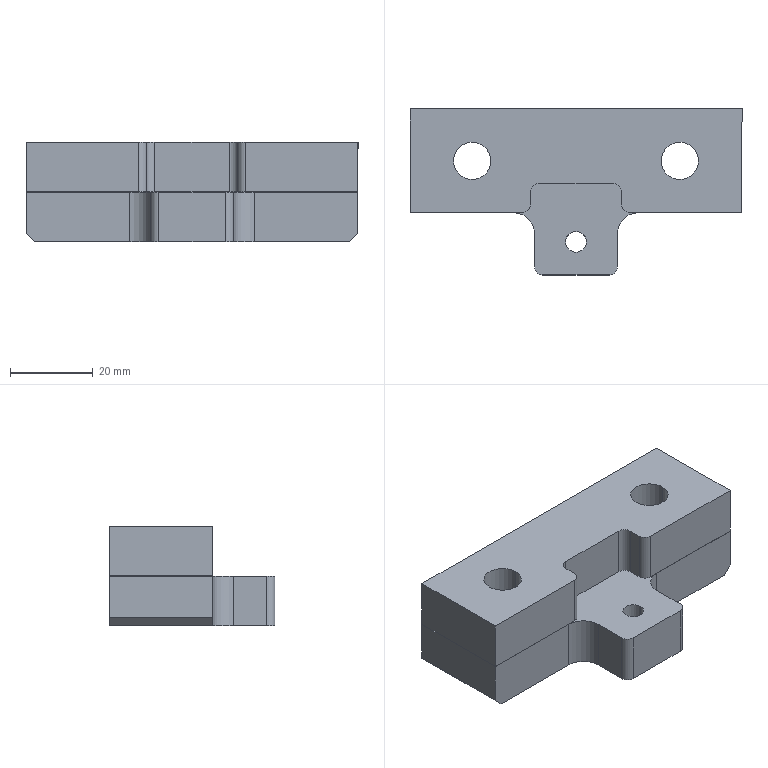Part | SolidWorks | features ICE 5, Fillet 3, HoleWzd 2, Chamfer 1, Extrusion 1 | 2 solids | 40 faces | box 80 x 40 x 24 mm | volume 46437 mm3 | plane 22 | cylinder 18 | commonest cylinder face diameters 9 x8 4 x6 5 x2 10 x2
STEP:
#1=CARTESIAN_POINT('',(60.5,7.5,-12.));
#2=VERTEX_POINT('',#1);
#3=CARTESIAN_POINT('',(69.5,7.5,-12.));
#4=VERTEX_POINT('',#3);
#5=CARTESIAN_POINT('',(65.,7.5,-12.));
#6=DIRECTION('',(0.,0.,1.));
#7=DIRECTION('',(-1.,0.,0.));
#8=AXIS2_PLACEMENT_3D('',#5,#6,#7);
#9=CIRCLE('',#8,4.5);
#10=EDGE_CURVE('',#2,#4,#9,.T.);
#11=ORIENTED_EDGE('',*,*,#10,.T.);
#12=CARTESIAN_POINT('',(69.5,7.5,-24.));
#13=VERTEX_POINT('',#12);
#14=CARTESIAN_POINT('',(69.5,7.5,-24.));
#15=DIRECTION('',(0.,0.,-1.));
#16=VECTOR('',#15,1000.);
#17=LINE('',#14,#16);
#18=EDGE_CURVE('',#4,#13,#17,.T.);
#19=ORIENTED_EDGE('',*,*,#18,.T.);
#20=CARTESIAN_POINT('',(60.5,7.5,-24.));
#21=VERTEX_POINT('',#20);
#22=CARTESIAN_POINT('',(65.,7.5,-24.));
#23=DIRECTION('',(0.,0.,-1.));
#24=DIRECTION('',(-1.,0.,0.));
#25=AXIS2_PLACEMENT_3D('',#22,#23,#24);
#26=CIRCLE('',#25,4.5);
#27=EDGE_CURVE('',#13,#21,#26,.T.);
#28=ORIENTED_EDGE('',*,*,#27,.T.);
#29=CARTESIAN_POINT('',(60.5,7.5,-24.));
#30=DIRECTION('',(0.,0.,-1.));
#31=VECTOR('',#30,1000.);
#32=LINE('',#29,#31);
#33=EDGE_CURVE('',#2,#21,#32,.T.);
#34=ORIENTED_EDGE('',*,*,#33,.F.);
#35=EDGE_LOOP('',(#11,#19,#28,#34));
#36=FACE_OUTER_BOUND('',#35,.T.);
#37=CARTESIAN_POINT('',(65.,7.5,-24.));
#38=DIRECTION('',(0.,0.,-1.));
#39=DIRECTION('',(-1.,0.,0.));
#40=AXIS2_PLACEMENT_3D('',#37,#38,#39);
#41=CYLINDRICAL_SURFACE('',#40,4.5);
#42=ADVANCED_FACE('',(#36),#41,.F.);
#43=CARTESIAN_POINT('',(10.5,7.5,-12.));
#44=VERTEX_POINT('',#43);
#45=CARTESIAN_POINT('',(19.5,7.5,-12.));
#46=VERTEX_POINT('',#45);
#47=CARTESIAN_POINT('',(15.,7.5,-12.));
#48=DIRECTION('',(0.,0.,1.));
#49=DIRECTION('',(-1.,0.,0.));
#50=AXIS2_PLACEMENT_3D('',#47,#48,#49);
#51=CIRCLE('',#50,4.5);
#52=EDGE_CURVE('',#44,#46,#51,.T.);
#53=ORIENTED_EDGE('',*,*,#52,.T.);
#54=CARTESIAN_POINT('',(19.5,7.5,-24.));
#55=VERTEX_POINT('',#54);
#56=CARTESIAN_POINT('',(19.5,7.5,-24.));
#57=DIRECTION('',(0.,0.,-1.));
#58=VECTOR('',#57,1000.);
#59=LINE('',#56,#58);
#60=EDGE_CURVE('',#46,#55,#59,.T.);
#61=ORIENTED_EDGE('',*,*,#60,.T.);
#62=CARTESIAN_POINT('',(10.5,7.5,-24.));
#63=VERTEX_POINT('',#62);
#64=CARTESIAN_POINT('',(15.,7.5,-24.));
#65=DIRECTION('',(0.,0.,-1.));
#66=DIRECTION('',(-1.,0.,0.));
#67=AXIS2_PLACEMENT_3D('',#64,#65,#66);
#68=CIRCLE('',#67,4.5);
#69=EDGE_CURVE('',#55,#63,#68,.T.);
#70=ORIENTED_EDGE('',*,*,#69,.T.);
#71=CARTESIAN_POINT('',(10.5,7.5,-24.));
#72=DIRECTION('',(0.,0.,-1.));
#73=VECTOR('',#72,1000.);
#74=LINE('',#71,#73);
#75=EDGE_CURVE('',#44,#63,#74,.T.);
#76=ORIENTED_EDGE('',*,*,#75,.F.);
#77=EDGE_LOOP('',(#53,#61,#70,#76));
#78=FACE_OUTER_BOUND('',#77,.T.);
#79=CARTESIAN_POINT('',(15.,7.5,-24.));
#80=DIRECTION('',(0.,0.,-1.));
#81=DIRECTION('',(-1.,0.,0.));
#82=AXIS2_PLACEMENT_3D('',#79,#80,#81);
#83=CYLINDRICAL_SURFACE('',#82,4.5);
#84=ADVANCED_FACE('',(#78),#83,.F.);
#85=CARTESIAN_POINT('',(37.5,-12.,-12.));
#86=VERTEX_POINT('',#85);
#87=CARTESIAN_POINT('',(42.5,-12.,-12.));
#88=VERTEX_POINT('',#87);
#89=CARTESIAN_POINT('',(40.,-12.,-12.));
#90=DIRECTION('',(0.,0.,1.));
#91=DIRECTION('',(1.,0.,0.));
#92=AXIS2_PLACEMENT_3D('',#89,#90,#91);
#93=CIRCLE('',#92,2.5);
#94=EDGE_CURVE('',#86,#88,#93,.T.);
#95=ORIENTED_EDGE('',*,*,#94,.T.);
#96=CARTESIAN_POINT('',(42.5,-12.,-24.));
#97=VERTEX_POINT('',#96);
#98=CARTESIAN_POINT('',(42.5,-12.,-24.));
#99=DIRECTION('',(0.,0.,-1.));
#100=VECTOR('',#99,1000.);
#101=LINE('',#98,#100);
#102=EDGE_CURVE('',#88,#97,#101,.T.);
#103=ORIENTED_EDGE('',*,*,#102,.T.);
#104=CARTESIAN_POINT('',(37.5,-12.,-24.));
#105=VERTEX_POINT('',#104);
#106=CARTESIAN_POINT('',(40.,-12.,-24.));
#107=DIRECTION('',(0.,0.,-1.));
#108=DIRECTION('',(-1.,0.,0.));
#109=AXIS2_PLACEMENT_3D('',#106,#107,#108);
#110=CIRCLE('',#109,2.5);
#111=EDGE_CURVE('',#97,#105,#110,.T.);
#112=ORIENTED_EDGE('',*,*,#111,.T.);
#113=CARTESIAN_POINT('',(37.5,-12.,-24.));
#114=DIRECTION('',(0.,0.,-1.));
#115=VECTOR('',#114,1000.);
#116=LINE('',#113,#115);
#117=EDGE_CURVE('',#86,#105,#116,.T.);
#118=ORIENTED_EDGE('',*,*,#117,.F.);
#119=EDGE_LOOP('',(#95,#103,#112,#118));
#120=FACE_OUTER_BOUND('',#119,.T.);
#121=CARTESIAN_POINT('',(40.,-12.,-24.));
#122=DIRECTION('',(0.,0.,-1.));
#123=DIRECTION('',(-1.,0.,0.));
#124=AXIS2_PLACEMENT_3D('',#121,#122,#123);
#125=CYLINDRICAL_SURFACE('',#124,2.5);
#126=ADVANCED_FACE('',(#120),#125,.F.);
#127=CARTESIAN_POINT('',(0.,-5.,-12.));
#128=VERTEX_POINT('',#127);
#129=CARTESIAN_POINT('',(25.,-5.,-12.));
#130=VERTEX_POINT('',#129);
#131=CARTESIAN_POINT('',(0.,-5.,-12.));
#132=DIRECTION('',(1.,0.,0.));
#133=VECTOR('',#132,1000.);
#134=LINE('',#131,#133);
#135=EDGE_CURVE('',#128,#130,#134,.T.);
#136=ORIENTED_EDGE('',*,*,#135,.T.);
#137=CARTESIAN_POINT('',(30.,-10.,-12.));
#138=VERTEX_POINT('',#137);
#139=CARTESIAN_POINT('',(25.,-10.,-12.));
#140=DIRECTION('',(0.,0.,-1.));
#141=DIRECTION('',(1.,0.,0.));
#142=AXIS2_PLACEMENT_3D('',#139,#140,#141);
#143=CIRCLE('',#142,5.);
#144=EDGE_CURVE('',#130,#138,#143,.T.);
#145=ORIENTED_EDGE('',*,*,#144,.T.);
#146=CARTESIAN_POINT('',(30.,-18.,-12.));
#147=VERTEX_POINT('',#146);
#148=CARTESIAN_POINT('',(30.,-5.,-12.));
#149=DIRECTION('',(0.,-1.,0.));
#150=VECTOR('',#149,1000.);
#151=LINE('',#148,#150);
#152=EDGE_CURVE('',#138,#147,#151,.T.);
#153=ORIENTED_EDGE('',*,*,#152,.T.);
#154=CARTESIAN_POINT('',(32.,-20.,-12.));
#155=VERTEX_POINT('',#154);
#156=CARTESIAN_POINT('',(32.,-18.,-12.));
#157=DIRECTION('',(0.,0.,1.));
#158=DIRECTION('',(1.,0.,0.));
#159=AXIS2_PLACEMENT_3D('',#156,#157,#158);
#160=CIRCLE('',#159,2.);
#161=EDGE_CURVE('',#147,#155,#160,.T.);
#162=ORIENTED_EDGE('',*,*,#161,.T.);
#163=CARTESIAN_POINT('',(48.,-20.,-12.));
#164=VERTEX_POINT('',#163);
#165=CARTESIAN_POINT('',(30.,-20.,-12.));
#166=DIRECTION('',(1.,0.,0.));
#167=VECTOR('',#166,1000.);
#168=LINE('',#165,#167);
#169=EDGE_CURVE('',#155,#164,#168,.T.);
#170=ORIENTED_EDGE('',*,*,#169,.T.);
#171=CARTESIAN_POINT('',(50.,-18.,-12.));
#172=VERTEX_POINT('',#171);
#173=CARTESIAN_POINT('',(48.,-18.,-12.));
#174=DIRECTION('',(0.,0.,1.));
#175=DIRECTION('',(1.,0.,0.));
#176=AXIS2_PLACEMENT_3D('',#173,#174,#175);
#177=CIRCLE('',#176,2.);
#178=EDGE_CURVE('',#164,#172,#177,.T.);
#179=ORIENTED_EDGE('',*,*,#178,.T.);
#180=CARTESIAN_POINT('',(50.,-10.,-12.));
#181=VERTEX_POINT('',#180);
#182=CARTESIAN_POINT('',(50.,-5.,-12.));
#183=DIRECTION('',(0.,1.,0.));
#184=VECTOR('',#183,1000.);
#185=LINE('',#182,#184);
#186=EDGE_CURVE('',#172,#181,#185,.T.);
#187=ORIENTED_EDGE('',*,*,#186,.T.);
#188=CARTESIAN_POINT('',(55.,-5.,-12.));
#189=VERTEX_POINT('',#188);
#190=CARTESIAN_POINT('',(55.,-10.,-12.));
#191=DIRECTION('',(0.,0.,-1.));
#192=DIRECTION('',(1.,0.,0.));
#193=AXIS2_PLACEMENT_3D('',#190,#191,#192);
#194=CIRCLE('',#193,5.);
#195=EDGE_CURVE('',#181,#189,#194,.T.);
#196=ORIENTED_EDGE('',*,*,#195,.T.);
#197=CARTESIAN_POINT('',(80.,-5.,-12.));
#198=VERTEX_POINT('',#197);
#199=CARTESIAN_POINT('',(0.,-5.,-12.));
#200=DIRECTION('',(1.,0.,0.));
#201=VECTOR('',#200,1000.);
#202=LINE('',#199,#201);
#203=EDGE_CURVE('',#189,#198,#202,.T.);
#204=ORIENTED_EDGE('',*,*,#203,.T.);
#205=CARTESIAN_POINT('',(80.,20.,-12.));
#206=VERTEX_POINT('',#205);
#207=CARTESIAN_POINT('',(80.,20.,-12.));
#208=DIRECTION('',(0.,-1.,0.));
#209=VECTOR('',#208,1000.);
#210=LINE('',#207,#209);
#211=EDGE_CURVE('',#206,#198,#210,.T.);
#212=ORIENTED_EDGE('',*,*,#211,.F.);
#213=CARTESIAN_POINT('',(0.,20.,-12.));
#214=VERTEX_POINT('',#213);
#215=CARTESIAN_POINT('',(0.,20.,-12.));
#216=DIRECTION('',(1.,0.,0.));
#217=VECTOR('',#216,1000.);
#218=LINE('',#215,#217);
#219=EDGE_CURVE('',#214,#206,#218,.T.);
#220=ORIENTED_EDGE('',*,*,#219,.F.);
#221=CARTESIAN_POINT('',(0.,20.,-12.));
#222=DIRECTION('',(0.,-1.,0.));
#223=VECTOR('',#222,1000.);
#224=LINE('',#221,#223);
#225=EDGE_CURVE('',#214,#128,#224,.T.);
#226=ORIENTED_EDGE('',*,*,#225,.T.);
#227=EDGE_LOOP('',(#136,#145,#153,#162,#170,#179,#187,#196,#204,#212,#220,#226));
#228=FACE_OUTER_BOUND('',#227,.T.);
#229=ORIENTED_EDGE('',*,*,#10,.F.);
#230=CARTESIAN_POINT('',(65.,7.5,-12.));
#231=DIRECTION('',(0.,0.,1.));
#232=DIRECTION('',(-1.,0.,0.));
#233=AXIS2_PLACEMENT_3D('',#230,#231,#232);
#234=CIRCLE('',#233,4.5);
#235=EDGE_CURVE('',#4,#2,#234,.T.);
#236=ORIENTED_EDGE('',*,*,#235,.F.);
#237=EDGE_LOOP('',(#229,#236));
#238=FACE_BOUND('',#237,.T.);
#239=ORIENTED_EDGE('',*,*,#52,.F.);
#240=CARTESIAN_POINT('',(15.,7.5,-12.));
#241=DIRECTION('',(0.,0.,1.));
#242=DIRECTION('',(-1.,0.,0.));
#243=AXIS2_PLACEMENT_3D('',#240,#241,#242);
#244=CIRCLE('',#243,4.5);
#245=EDGE_CURVE('',#46,#44,#244,.T.);
#246=ORIENTED_EDGE('',*,*,#245,.F.);
#247=EDGE_LOOP('',(#239,#246));
#248=FACE_BOUND('',#247,.T.);
#249=ORIENTED_EDGE('',*,*,#94,.F.);
#250=CARTESIAN_POINT('',(40.,-12.,-12.));
#251=DIRECTION('',(0.,0.,1.));
#252=DIRECTION('',(1.,0.,0.));
#253=AXIS2_PLACEMENT_3D('',#250,#251,#252);
#254=CIRCLE('',#253,2.5);
#255=EDGE_CURVE('',#88,#86,#254,.T.);
#256=ORIENTED_EDGE('',*,*,#255,.F.);
#257=EDGE_LOOP('',(#249,#256));
#258=FACE_BOUND('',#257,.T.);
#259=CARTESIAN_POINT('',(0.,0.,-12.));
#260=DIRECTION('',(0.,0.,1.));
#261=DIRECTION('',(1.,0.,0.));
#262=AXIS2_PLACEMENT_3D('',#259,#260,#261);
#263=PLANE('',#262);
#264=ADVANCED_FACE('',(#228,#238,#248,#258),#263,.T.);
#265=CARTESIAN_POINT('',(25.,-5.,-24.));
#266=VERTEX_POINT('',#265);
#267=CARTESIAN_POINT('',(25.,-5.,-12.));
#268=DIRECTION('',(0.,0.,1.));
#269=VECTOR('',#268,1000.);
#270=LINE('',#267,#269);
#271=EDGE_CURVE('',#266,#130,#270,.T.);
#272=ORIENTED_EDGE('',*,*,#271,.T.);
#273=ORIENTED_EDGE('',*,*,#135,.F.);
#274=CARTESIAN_POINT('',(0.,-5.,-22.));
#275=VERTEX_POINT('',#274);
#276=CARTESIAN_POINT('',(0.,-5.,0.));
#277=DIRECTION('',(0.,0.,-1.));
#278=VECTOR('',#277,1000.);
#279=LINE('',#276,#278);
#280=EDGE_CURVE('',#128,#275,#279,.T.);
#281=ORIENTED_EDGE('',*,*,#280,.T.);
#282=CARTESIAN_POINT('',(2.,-5.,-24.));
#283=VERTEX_POINT('',#282);
#284=CARTESIAN_POINT('',(0.,-5.,-22.));
#285=DIRECTION('',(0.7071,0.,-0.7071));
#286=VECTOR('',#285,1000.);
#287=LINE('',#284,#286);
#288=EDGE_CURVE('',#275,#283,#287,.T.);
#289=ORIENTED_EDGE('',*,*,#288,.T.);
#290=CARTESIAN_POINT('',(0.,-5.,-24.));
#291=DIRECTION('',(1.,0.,0.));
#292=VECTOR('',#291,1000.);
#293=LINE('',#290,#292);
#294=EDGE_CURVE('',#283,#266,#293,.T.);
#295=ORIENTED_EDGE('',*,*,#294,.T.);
#296=EDGE_LOOP('',(#272,#273,#281,#289,#295));
#297=FACE_OUTER_BOUND('',#296,.T.);
#298=CARTESIAN_POINT('',(30.,-5.,-12.));
#299=DIRECTION('',(0.,1.,0.));
#300=DIRECTION('',(-1.,0.,0.));
#301=AXIS2_PLACEMENT_3D('',#298,#299,#300);
#302=PLANE('',#301);
#303=ADVANCED_FACE('',(#297),#302,.F.);
#304=CARTESIAN_POINT('',(80.,20.,-22.));
#305=VERTEX_POINT('',#304);
#306=CARTESIAN_POINT('',(80.,20.,0.));
#307=DIRECTION('',(0.,0.,-1.));
#308=VECTOR('',#307,1000.);
#309=LINE('',#306,#308);
#310=EDGE_CURVE('',#206,#305,#309,.T.);
#311=ORIENTED_EDGE('',*,*,#310,.F.);
#312=ORIENTED_EDGE('',*,*,#211,.T.);
#313=CARTESIAN_POINT('',(80.,-5.,-22.));
#314=VERTEX_POINT('',#313);
#315=CARTESIAN_POINT('',(80.,-5.,0.));
#316=DIRECTION('',(0.,0.,-1.));
#317=VECTOR('',#316,1000.);
#318=LINE('',#315,#317);
#319=EDGE_CURVE('',#198,#314,#318,.T.);
#320=ORIENTED_EDGE('',*,*,#319,.T.);
#321=CARTESIAN_POINT('',(80.,20.,-22.));
#322=DIRECTION('',(0.,1.,0.));
#323=VECTOR('',#322,1000.);
#324=LINE('',#321,#323);
#325=EDGE_CURVE('',#314,#305,#324,.T.);
#326=ORIENTED_EDGE('',*,*,#325,.T.);
#327=EDGE_LOOP('',(#311,#312,#320,#326));
#328=FACE_OUTER_BOUND('',#327,.T.);
#329=CARTESIAN_POINT('',(80.,20.,0.));
#330=DIRECTION('',(-1.,0.,0.));
#331=DIRECTION('',(0.,0.,1.));
#332=AXIS2_PLACEMENT_3D('',#329,#330,#331);
#333=PLANE('',#332);
#334=ADVANCED_FACE('',(#328),#333,.F.);
#335=CARTESIAN_POINT('',(65.,7.5,-24.));
#336=DIRECTION('',(0.,0.,-1.));
#337=DIRECTION('',(-1.,0.,0.));
#338=AXIS2_PLACEMENT_3D('',#335,#336,#337);
#339=CIRCLE('',#338,4.5);
#340=EDGE_CURVE('',#21,#13,#339,.T.);
#341=ORIENTED_EDGE('',*,*,#340,.F.);
#342=ORIENTED_EDGE('',*,*,#27,.F.);
#343=EDGE_LOOP('',(#341,#342));
#344=FACE_BOUND('',#343,.T.);
#345=CARTESIAN_POINT('',(15.,7.5,-24.));
#346=DIRECTION('',(0.,0.,-1.));
#347=DIRECTION('',(-1.,0.,0.));
#348=AXIS2_PLACEMENT_3D('',#345,#346,#347);
#349=CIRCLE('',#348,4.5);
#350=EDGE_CURVE('',#63,#55,#349,.T.);
#351=ORIENTED_EDGE('',*,*,#350,.F.);
#352=ORIENTED_EDGE('',*,*,#69,.F.);
#353=EDGE_LOOP('',(#351,#352));
#354=FACE_BOUND('',#353,.T.);
#355=CARTESIAN_POINT('',(40.,-12.,-24.));
#356=DIRECTION('',(0.,0.,-1.));
#357=DIRECTION('',(-1.,0.,0.));
#358=AXIS2_PLACEMENT_3D('',#355,#356,#357);
#359=CIRCLE('',#358,2.5);
#360=EDGE_CURVE('',#105,#97,#359,.T.);
#361=ORIENTED_EDGE('',*,*,#360,.F.);
#362=ORIENTED_EDGE('',*,*,#111,.F.);
#363=EDGE_LOOP('',(#361,#362));
#364=FACE_BOUND('',#363,.T.);
#365=CARTESIAN_POINT('',(50.,-18.,-24.));
#366=VERTEX_POINT('',#365);
#367=CARTESIAN_POINT('',(50.,-10.,-24.));
#368=VERTEX_POINT('',#367);
#369=CARTESIAN_POINT('',(50.,-20.,-24.));
#370=DIRECTION('',(0.,1.,0.));
#371=VECTOR('',#370,1000.);
#372=LINE('',#369,#371);
#373=EDGE_CURVE('',#366,#368,#372,.T.);
#374=ORIENTED_EDGE('',*,*,#373,.F.);
#375=CARTESIAN_POINT('',(48.,-20.,-24.));
#376=VERTEX_POINT('',#375);
#377=CARTESIAN_POINT('',(48.,-18.,-24.));
#378=DIRECTION('',(0.,0.,-1.));
#379=DIRECTION('',(1.,0.,0.));
#380=AXIS2_PLACEMENT_3D('',#377,#378,#379);
#381=CIRCLE('',#380,2.);
#382=EDGE_CURVE('',#366,#376,#381,.T.);
#383=ORIENTED_EDGE('',*,*,#382,.T.);
#384=CARTESIAN_POINT('',(32.,-20.,-24.));
#385=VERTEX_POINT('',#384);
#386=CARTESIAN_POINT('',(80.,-20.,-24.));
#387=DIRECTION('',(-1.,0.,0.));
#388=VECTOR('',#387,1000.);
#389=LINE('',#386,#388);
#390=EDGE_CURVE('',#376,#385,#389,.T.);
#391=ORIENTED_EDGE('',*,*,#390,.T.);
#392=CARTESIAN_POINT('',(30.,-18.,-24.));
#393=VERTEX_POINT('',#392);
#394=CARTESIAN_POINT('',(32.,-18.,-24.));
#395=DIRECTION('',(0.,0.,-1.));
#396=DIRECTION('',(1.,0.,0.));
#397=AXIS2_PLACEMENT_3D('',#394,#395,#396);
#398=CIRCLE('',#397,2.);
#399=EDGE_CURVE('',#385,#393,#398,.T.);
#400=ORIENTED_EDGE('',*,*,#399,.T.);
#401=CARTESIAN_POINT('',(30.,-10.,-24.));
#402=VERTEX_POINT('',#401);
#403=CARTESIAN_POINT('',(30.,-20.,-24.));
#404=DIRECTION('',(0.,-1.,0.));
#405=VECTOR('',#404,1000.);
#406=LINE('',#403,#405);
#407=EDGE_CURVE('',#402,#393,#406,.T.);
#408=ORIENTED_EDGE('',*,*,#407,.F.);
#409=CARTESIAN_POINT('',(25.,-10.,-24.));
#410=DIRECTION('',(0.,0.,1.));
#411=DIRECTION('',(1.,0.,0.));
#412=AXIS2_PLACEMENT_3D('',#409,#410,#411);
#413=CIRCLE('',#412,5.);
#414=EDGE_CURVE('',#402,#266,#413,.T.);
#415=ORIENTED_EDGE('',*,*,#414,.T.);
#416=ORIENTED_EDGE('',*,*,#294,.F.);
#417=CARTESIAN_POINT('',(2.,20.,-24.));
#418=VERTEX_POINT('',#417);
#419=CARTESIAN_POINT('',(2.,20.,-24.));
#420=DIRECTION('',(0.,1.,0.));
#421=VECTOR('',#420,1000.);
#422=LINE('',#419,#421);
#423=EDGE_CURVE('',#283,#418,#422,.T.);
#424=ORIENTED_EDGE('',*,*,#423,.T.);
#425=CARTESIAN_POINT('',(78.,20.,-24.));
#426=VERTEX_POINT('',#425);
#427=CARTESIAN_POINT('',(80.,20.,-24.));
#428=DIRECTION('',(-1.,0.,0.));
#429=VECTOR('',#428,1000.);
#430=LINE('',#427,#429);
#431=EDGE_CURVE('',#426,#418,#430,.T.);
#432=ORIENTED_EDGE('',*,*,#431,.F.);
#433=CARTESIAN_POINT('',(78.,-5.,-24.));
#434=VERTEX_POINT('',#433);
#435=CARTESIAN_POINT('',(78.,20.,-24.));
#436=DIRECTION('',(0.,-1.,0.));
#437=VECTOR('',#436,1000.);
#438=LINE('',#435,#437);
#439=EDGE_CURVE('',#426,#434,#438,.T.);
#440=ORIENTED_EDGE('',*,*,#439,.T.);
#441=CARTESIAN_POINT('',(55.,-5.,-24.));
#442=VERTEX_POINT('',#441);
#443=CARTESIAN_POINT('',(80.,-5.,-24.));
#444=DIRECTION('',(1.,0.,0.));
#445=VECTOR('',#444,1000.);
#446=LINE('',#443,#445);
#447=EDGE_CURVE('',#442,#434,#446,.T.);
#448=ORIENTED_EDGE('',*,*,#447,.F.);
#449=CARTESIAN_POINT('',(55.,-10.,-24.));
#450=DIRECTION('',(0.,0.,1.));
#451=DIRECTION('',(1.,0.,0.));
#452=AXIS2_PLACEMENT_3D('',#449,#450,#451);
#453=CIRCLE('',#452,5.);
#454=EDGE_CURVE('',#442,#368,#453,.T.);
#455=ORIENTED_EDGE('',*,*,#454,.T.);
#456=EDGE_LOOP('',(#374,#383,#391,#400,#408,#415,#416,#424,#432,#440,#448,#455));
#457=FACE_OUTER_BOUND('',#456,.T.);
#458=CARTESIAN_POINT('',(80.,20.,-24.));
#459=DIRECTION('',(0.,0.,1.));
#460=DIRECTION('',(1.,0.,0.));
#461=AXIS2_PLACEMENT_3D('',#458,#459,#460);
#462=PLANE('',#461);
#463=ADVANCED_FACE('',(#344,#354,#364,#457),#462,.F.);
#464=ORIENTED_EDGE('',*,*,#280,.F.);
#465=ORIENTED_EDGE('',*,*,#225,.F.);
#466=CARTESIAN_POINT('',(0.,20.,-22.));
#467=VERTEX_POINT('',#466);
#468=CARTESIAN_POINT('',(0.,20.,-24.));
#469=DIRECTION('',(0.,0.,1.));
#470=VECTOR('',#469,1000.);
#471=LINE('',#468,#470);
#472=EDGE_CURVE('',#467,#214,#471,.T.);
#473=ORIENTED_EDGE('',*,*,#472,.F.);
#474=CARTESIAN_POINT('',(0.,20.,-22.));
#475=DIRECTION('',(0.,-1.,0.));
#476=VECTOR('',#475,1000.);
#477=LINE('',#474,#476);
#478=EDGE_CURVE('',#467,#275,#477,.T.);
#479=ORIENTED_EDGE('',*,*,#478,.T.);
#480=EDGE_LOOP('',(#464,#465,#473,#479));
#481=FACE_OUTER_BOUND('',#480,.T.);
#482=CARTESIAN_POINT('',(0.,20.,-24.));
#483=DIRECTION('',(1.,0.,0.));
#484=DIRECTION('',(0.,0.,-1.));
#485=AXIS2_PLACEMENT_3D('',#482,#483,#484);
#486=PLANE('',#485);
#487=ADVANCED_FACE('',(#481),#486,.F.);
#488=ORIENTED_EDGE('',*,*,#219,.T.);
#489=ORIENTED_EDGE('',*,*,#310,.T.);
#490=CARTESIAN_POINT('',(51.,20.,-51.));
#491=DIRECTION('',(-0.7071,0.,-0.7071));
#492=VECTOR('',#491,1000.);
#493=LINE('',#490,#492);
#494=EDGE_CURVE('',#305,#426,#493,.T.);
#495=ORIENTED_EDGE('',*,*,#494,.T.);
#496=ORIENTED_EDGE('',*,*,#431,.T.);
#497=CARTESIAN_POINT('',(-11.,20.,-11.));
#498=DIRECTION('',(-0.7071,0.,0.7071));
#499=VECTOR('',#498,1000.);
#500=LINE('',#497,#499);
#501=EDGE_CURVE('',#418,#467,#500,.T.);
#502=ORIENTED_EDGE('',*,*,#501,.T.);
#503=ORIENTED_EDGE('',*,*,#472,.T.);
#504=EDGE_LOOP('',(#488,#489,#495,#496,#502,#503));
#505=FACE_OUTER_BOUND('',#504,.T.);
#506=CARTESIAN_POINT('',(0.,20.,0.));
#507=DIRECTION('',(0.,1.,0.));
#508=DIRECTION('',(0.,0.,1.));
#509=AXIS2_PLACEMENT_3D('',#506,#507,#508);
#510=PLANE('',#509);
#511=ADVANCED_FACE('',(#505),#510,.T.);
#512=ORIENTED_EDGE('',*,*,#390,.F.);
#513=CARTESIAN_POINT('',(48.,-20.,0.));
#514=DIRECTION('',(0.,0.,1.));
#515=VECTOR('',#514,1000.);
#516=LINE('',#513,#515);
#517=EDGE_CURVE('',#376,#164,#516,.T.);
#518=ORIENTED_EDGE('',*,*,#517,.T.);
#519=ORIENTED_EDGE('',*,*,#169,.F.);
#520=CARTESIAN_POINT('',(32.,-20.,0.));
#521=DIRECTION('',(0.,0.,-1.));
#522=VECTOR('',#521,1000.);
#523=LINE('',#520,#522);
#524=EDGE_CURVE('',#155,#385,#523,.T.);
#525=ORIENTED_EDGE('',*,*,#524,.T.);
#526=EDGE_LOOP('',(#512,#518,#519,#525));
#527=FACE_OUTER_BOUND('',#526,.T.);
#528=CARTESIAN_POINT('',(0.,-20.,0.));
#529=DIRECTION('',(0.,1.,0.));
#530=DIRECTION('',(0.,0.,1.));
#531=AXIS2_PLACEMENT_3D('',#528,#529,#530);
#532=PLANE('',#531);
#533=ADVANCED_FACE('',(#527),#532,.F.);
#534=ORIENTED_EDGE('',*,*,#288,.F.);
#535=ORIENTED_EDGE('',*,*,#478,.F.);
#536=ORIENTED_EDGE('',*,*,#501,.F.);
#537=ORIENTED_EDGE('',*,*,#423,.F.);
#538=EDGE_LOOP('',(#534,#535,#536,#537));
#539=FACE_OUTER_BOUND('',#538,.T.);
#540=CARTESIAN_POINT('',(0.,20.,-22.));
#541=DIRECTION('',(0.7071,0.,0.7071));
#542=DIRECTION('',(0.,-1.,0.));
#543=AXIS2_PLACEMENT_3D('',#540,#541,#542);
#544=PLANE('',#543);
#545=ADVANCED_FACE('',(#539),#544,.F.);
#546=CARTESIAN_POINT('',(78.,-5.,-24.));
#547=DIRECTION('',(0.7071,0.,0.7071));
#548=VECTOR('',#547,1000.);
#549=LINE('',#546,#548);
#550=EDGE_CURVE('',#434,#314,#549,.T.);
#551=ORIENTED_EDGE('',*,*,#550,.F.);
#552=ORIENTED_EDGE('',*,*,#439,.F.);
#553=ORIENTED_EDGE('',*,*,#494,.F.);
#554=ORIENTED_EDGE('',*,*,#325,.F.);
#555=EDGE_LOOP('',(#551,#552,#553,#554));
#556=FACE_OUTER_BOUND('',#555,.T.);
#557=CARTESIAN_POINT('',(78.,20.,-24.));
#558=DIRECTION('',(-0.7071,0.,0.7071));
#559=DIRECTION('',(0.,-1.,0.));
#560=AXIS2_PLACEMENT_3D('',#557,#558,#559);
#561=PLANE('',#560);
#562=ADVANCED_FACE('',(#556),#561,.F.);
#563=ORIENTED_EDGE('',*,*,#319,.F.);
#564=ORIENTED_EDGE('',*,*,#203,.F.);
#565=CARTESIAN_POINT('',(55.,-5.,-24.));
#566=DIRECTION('',(0.,0.,-1.));
#567=VECTOR('',#566,1000.);
#568=LINE('',#565,#567);
#569=EDGE_CURVE('',#189,#442,#568,.T.);
#570=ORIENTED_EDGE('',*,*,#569,.T.);
#571=ORIENTED_EDGE('',*,*,#447,.T.);
#572=ORIENTED_EDGE('',*,*,#550,.T.);
#573=EDGE_LOOP('',(#563,#564,#570,#571,#572));
#574=FACE_OUTER_BOUND('',#573,.T.);
#575=CARTESIAN_POINT('',(30.,-5.,-12.));
#576=DIRECTION('',(0.,1.,0.));
#577=DIRECTION('',(-1.,0.,0.));
#578=AXIS2_PLACEMENT_3D('',#575,#576,#577);
#579=PLANE('',#578);
#580=ADVANCED_FACE('',(#574),#579,.F.);
#581=ORIENTED_EDGE('',*,*,#102,.F.);
#582=ORIENTED_EDGE('',*,*,#255,.T.);
#583=ORIENTED_EDGE('',*,*,#117,.T.);
#584=ORIENTED_EDGE('',*,*,#360,.T.);
#585=EDGE_LOOP('',(#581,#582,#583,#584));
#586=FACE_OUTER_BOUND('',#585,.T.);
#587=CARTESIAN_POINT('',(40.,-12.,-24.));
#588=DIRECTION('',(0.,0.,-1.));
#589=DIRECTION('',(-1.,0.,0.));
#590=AXIS2_PLACEMENT_3D('',#587,#588,#589);
#591=CYLINDRICAL_SURFACE('',#590,2.5);
#592=ADVANCED_FACE('',(#586),#591,.F.);
#593=ORIENTED_EDGE('',*,*,#60,.F.);
#594=ORIENTED_EDGE('',*,*,#245,.T.);
#595=ORIENTED_EDGE('',*,*,#75,.T.);
#596=ORIENTED_EDGE('',*,*,#350,.T.);
#597=EDGE_LOOP('',(#593,#594,#595,#596));
#598=FACE_OUTER_BOUND('',#597,.T.);
#599=CARTESIAN_POINT('',(15.,7.5,-24.));
#600=DIRECTION('',(0.,0.,-1.));
#601=DIRECTION('',(-1.,0.,0.));
#602=AXIS2_PLACEMENT_3D('',#599,#600,#601);
#603=CYLINDRICAL_SURFACE('',#602,4.5);
#604=ADVANCED_FACE('',(#598),#603,.F.);
#605=ORIENTED_EDGE('',*,*,#18,.F.);
#606=ORIENTED_EDGE('',*,*,#235,.T.);
#607=ORIENTED_EDGE('',*,*,#33,.T.);
#608=ORIENTED_EDGE('',*,*,#340,.T.);
#609=EDGE_LOOP('',(#605,#606,#607,#608));
#610=FACE_OUTER_BOUND('',#609,.T.);
#611=CARTESIAN_POINT('',(65.,7.5,-24.));
#612=DIRECTION('',(0.,0.,-1.));
#613=DIRECTION('',(-1.,0.,0.));
#614=AXIS2_PLACEMENT_3D('',#611,#612,#613);
#615=CYLINDRICAL_SURFACE('',#614,4.5);
#616=ADVANCED_FACE('',(#610),#615,.F.);
#617=ORIENTED_EDGE('',*,*,#407,.T.);
#618=CARTESIAN_POINT('',(30.,-18.,0.));
#619=DIRECTION('',(0.,0.,1.));
#620=VECTOR('',#619,1000.);
#621=LINE('',#618,#620);
#622=EDGE_CURVE('',#393,#147,#621,.T.);
#623=ORIENTED_EDGE('',*,*,#622,.T.);
#624=ORIENTED_EDGE('',*,*,#152,.F.);
#625=CARTESIAN_POINT('',(30.,-10.,-24.));
#626=DIRECTION('',(0.,0.,-1.));
#627=VECTOR('',#626,1000.);
#628=LINE('',#625,#627);
#629=EDGE_CURVE('',#138,#402,#628,.T.);
#630=ORIENTED_EDGE('',*,*,#629,.T.);
#631=EDGE_LOOP('',(#617,#623,#624,#630));
#632=FACE_OUTER_BOUND('',#631,.T.);
#633=CARTESIAN_POINT('',(30.,-20.,0.));
#634=DIRECTION('',(1.,0.,0.));
#635=DIRECTION('',(0.,1.,0.));
#636=AXIS2_PLACEMENT_3D('',#633,#634,#635);
#637=PLANE('',#636);
#638=ADVANCED_FACE('',(#632),#637,.F.);
#639=ORIENTED_EDGE('',*,*,#186,.F.);
#640=CARTESIAN_POINT('',(50.,-18.,0.));
#641=DIRECTION('',(0.,0.,-1.));
#642=VECTOR('',#641,1000.);
#643=LINE('',#640,#642);
#644=EDGE_CURVE('',#172,#366,#643,.T.);
#645=ORIENTED_EDGE('',*,*,#644,.T.);
#646=ORIENTED_EDGE('',*,*,#373,.T.);
#647=CARTESIAN_POINT('',(50.,-10.,-12.));
#648=DIRECTION('',(0.,0.,1.));
#649=VECTOR('',#648,1000.);
#650=LINE('',#647,#649);
#651=EDGE_CURVE('',#368,#181,#650,.T.);
#652=ORIENTED_EDGE('',*,*,#651,.T.);
#653=EDGE_LOOP('',(#639,#645,#646,#652));
#654=FACE_OUTER_BOUND('',#653,.T.);
#655=CARTESIAN_POINT('',(50.,-20.,0.));
#656=DIRECTION('',(-1.,0.,0.));
#657=DIRECTION('',(0.,0.,1.));
#658=AXIS2_PLACEMENT_3D('',#655,#656,#657);
#659=PLANE('',#658);
#660=ADVANCED_FACE('',(#654),#659,.F.);
#661=ORIENTED_EDGE('',*,*,#195,.F.);
#662=ORIENTED_EDGE('',*,*,#651,.F.);
#663=ORIENTED_EDGE('',*,*,#454,.F.);
#664=ORIENTED_EDGE('',*,*,#569,.F.);
#665=EDGE_LOOP('',(#661,#662,#663,#664));
#666=FACE_OUTER_BOUND('',#665,.T.);
#667=CARTESIAN_POINT('',(55.,-10.,-12.));
#668=DIRECTION('',(0.,0.,1.));
#669=DIRECTION('',(1.,0.,0.));
#670=AXIS2_PLACEMENT_3D('',#667,#668,#669);
#671=CYLINDRICAL_SURFACE('',#670,5.);
#672=ADVANCED_FACE('',(#666),#671,.F.);
#673=ORIENTED_EDGE('',*,*,#144,.F.);
#674=ORIENTED_EDGE('',*,*,#271,.F.);
#675=ORIENTED_EDGE('',*,*,#414,.F.);
#676=ORIENTED_EDGE('',*,*,#629,.F.);
#677=EDGE_LOOP('',(#673,#674,#675,#676));
#678=FACE_OUTER_BOUND('',#677,.T.);
#679=CARTESIAN_POINT('',(25.,-10.,0.));
#680=DIRECTION('',(0.,0.,1.));
#681=DIRECTION('',(1.,0.,0.));
#682=AXIS2_PLACEMENT_3D('',#679,#680,#681);
#683=CYLINDRICAL_SURFACE('',#682,5.);
#684=ADVANCED_FACE('',(#678),#683,.F.);
#685=ORIENTED_EDGE('',*,*,#178,.F.);
#686=ORIENTED_EDGE('',*,*,#517,.F.);
#687=ORIENTED_EDGE('',*,*,#382,.F.);
#688=ORIENTED_EDGE('',*,*,#644,.F.);
#689=EDGE_LOOP('',(#685,#686,#687,#688));
#690=FACE_OUTER_BOUND('',#689,.T.);
#691=CARTESIAN_POINT('',(48.,-18.,0.));
#692=DIRECTION('',(0.,0.,-1.));
#693=DIRECTION('',(-1.,0.,0.));
#694=AXIS2_PLACEMENT_3D('',#691,#692,#693);
#695=CYLINDRICAL_SURFACE('',#694,2.);
#696=ADVANCED_FACE('',(#690),#695,.T.);
#697=ORIENTED_EDGE('',*,*,#161,.F.);
#698=ORIENTED_EDGE('',*,*,#622,.F.);
#699=ORIENTED_EDGE('',*,*,#399,.F.);
#700=ORIENTED_EDGE('',*,*,#524,.F.);
#701=EDGE_LOOP('',(#697,#698,#699,#700));
#702=FACE_OUTER_BOUND('',#701,.T.);
#703=CARTESIAN_POINT('',(32.,-18.,0.));
#704=DIRECTION('',(0.,0.,-1.));
#705=DIRECTION('',(-1.,0.,0.));
#706=AXIS2_PLACEMENT_3D('',#703,#704,#705);
#707=CYLINDRICAL_SURFACE('',#706,2.);
#708=ADVANCED_FACE('',(#702),#707,.T.);
#709=CLOSED_SHELL('',(#42,#84,#126,#264,#303,#334,#463,#487,#511,#533,#545,#562,#580,#592,#604,#616,#638,#660,#672,#684,#696,#708));
#710=MANIFOLD_SOLID_BREP('',#709);
#711=CARTESIAN_POINT('',(69.5,7.5,0.));
#712=VERTEX_POINT('',#711);
#713=CARTESIAN_POINT('',(60.5,7.5,0.));
#714=VERTEX_POINT('',#713);
#715=CARTESIAN_POINT('',(65.,7.5,0.));
#716=DIRECTION('',(0.,0.,-1.));
#717=DIRECTION('',(-1.,0.,0.));
#718=AXIS2_PLACEMENT_3D('',#715,#716,#717);
#719=CIRCLE('',#718,4.5);
#720=EDGE_CURVE('',#712,#714,#719,.T.);
#721=ORIENTED_EDGE('',*,*,#720,.F.);
#722=CARTESIAN_POINT('',(69.5,7.5,-11.98));
#723=VERTEX_POINT('',#722);
#724=CARTESIAN_POINT('',(69.5,7.5,-24.));
#725=DIRECTION('',(0.,0.,-1.));
#726=VECTOR('',#725,1000.);
#727=LINE('',#724,#726);
#728=EDGE_CURVE('',#712,#723,#727,.T.);
#729=ORIENTED_EDGE('',*,*,#728,.T.);
#730=CARTESIAN_POINT('',(60.5,7.5,-11.98));
#731=VERTEX_POINT('',#730);
#732=CARTESIAN_POINT('',(65.,7.5,-11.98));
#733=DIRECTION('',(0.,0.,-1.));
#734=DIRECTION('',(1.,0.,0.));
#735=AXIS2_PLACEMENT_3D('',#732,#733,#734);
#736=CIRCLE('',#735,4.5);
#737=EDGE_CURVE('',#723,#731,#736,.T.);
#738=ORIENTED_EDGE('',*,*,#737,.T.);
#739=CARTESIAN_POINT('',(60.5,7.5,-24.));
#740=DIRECTION('',(0.,0.,-1.));
#741=VECTOR('',#740,1000.);
#742=LINE('',#739,#741);
#743=EDGE_CURVE('',#714,#731,#742,.T.);
#744=ORIENTED_EDGE('',*,*,#743,.F.);
#745=EDGE_LOOP('',(#721,#729,#738,#744));
#746=FACE_OUTER_BOUND('',#745,.T.);
#747=CARTESIAN_POINT('',(65.,7.5,-24.));
#748=DIRECTION('',(0.,0.,-1.));
#749=DIRECTION('',(-1.,0.,0.));
#750=AXIS2_PLACEMENT_3D('',#747,#748,#749);
#751=CYLINDRICAL_SURFACE('',#750,4.5);
#752=ADVANCED_FACE('',(#746),#751,.F.);
#753=CARTESIAN_POINT('',(19.5,7.5,0.));
#754=VERTEX_POINT('',#753);
#755=CARTESIAN_POINT('',(10.5,7.5,0.));
#756=VERTEX_POINT('',#755);
#757=CARTESIAN_POINT('',(15.,7.5,0.));
#758=DIRECTION('',(0.,0.,-1.));
#759=DIRECTION('',(-1.,0.,0.));
#760=AXIS2_PLACEMENT_3D('',#757,#758,#759);
#761=CIRCLE('',#760,4.5);
#762=EDGE_CURVE('',#754,#756,#761,.T.);
#763=ORIENTED_EDGE('',*,*,#762,.F.);
#764=CARTESIAN_POINT('',(19.5,7.5,-11.98));
#765=VERTEX_POINT('',#764);
#766=CARTESIAN_POINT('',(19.5,7.5,-24.));
#767=DIRECTION('',(0.,0.,-1.));
#768=VECTOR('',#767,1000.);
#769=LINE('',#766,#768);
#770=EDGE_CURVE('',#754,#765,#769,.T.);
#771=ORIENTED_EDGE('',*,*,#770,.T.);
#772=CARTESIAN_POINT('',(10.5,7.5,-11.98));
#773=VERTEX_POINT('',#772);
#774=CARTESIAN_POINT('',(15.,7.5,-11.98));
#775=DIRECTION('',(0.,0.,-1.));
#776=DIRECTION('',(1.,0.,0.));
#777=AXIS2_PLACEMENT_3D('',#774,#775,#776);
#778=CIRCLE('',#777,4.5);
#779=EDGE_CURVE('',#765,#773,#778,.T.);
#780=ORIENTED_EDGE('',*,*,#779,.T.);
#781=CARTESIAN_POINT('',(10.5,7.5,-24.));
#782=DIRECTION('',(0.,0.,-1.));
#783=VECTOR('',#782,1000.);
#784=LINE('',#781,#783);
#785=EDGE_CURVE('',#756,#773,#784,.T.);
#786=ORIENTED_EDGE('',*,*,#785,.F.);
#787=EDGE_LOOP('',(#763,#771,#780,#786));
#788=FACE_OUTER_BOUND('',#787,.T.);
#789=CARTESIAN_POINT('',(15.,7.5,-24.));
#790=DIRECTION('',(0.,0.,-1.));
#791=DIRECTION('',(-1.,0.,0.));
#792=AXIS2_PLACEMENT_3D('',#789,#790,#791);
#793=CYLINDRICAL_SURFACE('',#792,4.5);
#794=ADVANCED_FACE('',(#788),#793,.F.);
#795=ORIENTED_EDGE('',*,*,#770,.F.);
#796=CARTESIAN_POINT('',(15.,7.5,0.));
#797=DIRECTION('',(0.,0.,-1.));
#798=DIRECTION('',(-1.,0.,0.));
#799=AXIS2_PLACEMENT_3D('',#796,#797,#798);
#800=CIRCLE('',#799,4.5);
#801=EDGE_CURVE('',#756,#754,#800,.T.);
#802=ORIENTED_EDGE('',*,*,#801,.F.);
#803=ORIENTED_EDGE('',*,*,#785,.T.);
#804=CARTESIAN_POINT('',(15.,7.5,-11.98));
#805=DIRECTION('',(0.,0.,-1.));
#806=DIRECTION('',(1.,0.,0.));
#807=AXIS2_PLACEMENT_3D('',#804,#805,#806);
#808=CIRCLE('',#807,4.5);
#809=EDGE_CURVE('',#773,#765,#808,.T.);
#810=ORIENTED_EDGE('',*,*,#809,.T.);
#811=EDGE_LOOP('',(#795,#802,#803,#810));
#812=FACE_OUTER_BOUND('',#811,.T.);
#813=CARTESIAN_POINT('',(15.,7.5,-24.));
#814=DIRECTION('',(0.,0.,-1.));
#815=DIRECTION('',(-1.,0.,0.));
#816=AXIS2_PLACEMENT_3D('',#813,#814,#815);
#817=CYLINDRICAL_SURFACE('',#816,4.5);
#818=ADVANCED_FACE('',(#812),#817,.F.);
#819=ORIENTED_EDGE('',*,*,#728,.F.);
#820=CARTESIAN_POINT('',(65.,7.5,0.));
#821=DIRECTION('',(0.,0.,-1.));
#822=DIRECTION('',(-1.,0.,0.));
#823=AXIS2_PLACEMENT_3D('',#820,#821,#822);
#824=CIRCLE('',#823,4.5);
#825=EDGE_CURVE('',#714,#712,#824,.T.);
#826=ORIENTED_EDGE('',*,*,#825,.F.);
#827=ORIENTED_EDGE('',*,*,#743,.T.);
#828=CARTESIAN_POINT('',(65.,7.5,-11.98));
#829=DIRECTION('',(0.,0.,-1.));
#830=DIRECTION('',(1.,0.,0.));
#831=AXIS2_PLACEMENT_3D('',#828,#829,#830);
#832=CIRCLE('',#831,4.5);
#833=EDGE_CURVE('',#731,#723,#832,.T.);
#834=ORIENTED_EDGE('',*,*,#833,.T.);
#835=EDGE_LOOP('',(#819,#826,#827,#834));
#836=FACE_OUTER_BOUND('',#835,.T.);
#837=CARTESIAN_POINT('',(65.,7.5,-24.));
#838=DIRECTION('',(0.,0.,-1.));
#839=DIRECTION('',(-1.,0.,0.));
#840=AXIS2_PLACEMENT_3D('',#837,#838,#839);
#841=CYLINDRICAL_SURFACE('',#840,4.5);
#842=ADVANCED_FACE('',(#836),#841,.F.);
#843=ORIENTED_EDGE('',*,*,#825,.T.);
#844=ORIENTED_EDGE('',*,*,#720,.T.);
#845=EDGE_LOOP('',(#843,#844));
#846=FACE_BOUND('',#845,.T.);
#847=ORIENTED_EDGE('',*,*,#801,.T.);
#848=ORIENTED_EDGE('',*,*,#762,.T.);
#849=EDGE_LOOP('',(#847,#848));
#850=FACE_BOUND('',#849,.T.);
#851=CARTESIAN_POINT('',(27.,-5.,0.));
#852=VERTEX_POINT('',#851);
#853=CARTESIAN_POINT('',(0.,-5.,0.));
#854=VERTEX_POINT('',#853);
#855=CARTESIAN_POINT('',(30.,-5.,0.));
#856=DIRECTION('',(-1.,0.,0.));
#857=VECTOR('',#856,1000.);
#858=LINE('',#855,#857);
#859=EDGE_CURVE('',#852,#854,#858,.T.);
#860=ORIENTED_EDGE('',*,*,#859,.F.);
#861=CARTESIAN_POINT('',(29.,-3.,0.));
#862=VERTEX_POINT('',#861);
#863=CARTESIAN_POINT('',(27.,-3.,0.));
#864=DIRECTION('',(0.,0.,1.));
#865=DIRECTION('',(-1.,0.,0.));
#866=AXIS2_PLACEMENT_3D('',#863,#864,#865);
#867=CIRCLE('',#866,2.);
#868=EDGE_CURVE('',#852,#862,#867,.T.);
#869=ORIENTED_EDGE('',*,*,#868,.T.);
#870=CARTESIAN_POINT('',(29.,0.,0.));
#871=VERTEX_POINT('',#870);
#872=CARTESIAN_POINT('',(29.,-5.,0.));
#873=DIRECTION('',(0.,-1.,0.));
#874=VECTOR('',#873,1000.);
#875=LINE('',#872,#874);
#876=EDGE_CURVE('',#871,#862,#875,.T.);
#877=ORIENTED_EDGE('',*,*,#876,.F.);
#878=CARTESIAN_POINT('',(31.,2.,0.));
#879=VERTEX_POINT('',#878);
#880=CARTESIAN_POINT('',(31.,0.,0.));
#881=DIRECTION('',(0.,0.,-1.));
#882=DIRECTION('',(-1.,0.,0.));
#883=AXIS2_PLACEMENT_3D('',#880,#881,#882);
#884=CIRCLE('',#883,2.);
#885=EDGE_CURVE('',#871,#879,#884,.T.);
#886=ORIENTED_EDGE('',*,*,#885,.T.);
#887=CARTESIAN_POINT('',(49.,2.,0.));
#888=VERTEX_POINT('',#887);
#889=CARTESIAN_POINT('',(29.,2.,0.));
#890=DIRECTION('',(-1.,0.,0.));
#891=VECTOR('',#890,1000.);
#892=LINE('',#889,#891);
#893=EDGE_CURVE('',#888,#879,#892,.T.);
#894=ORIENTED_EDGE('',*,*,#893,.F.);
#895=CARTESIAN_POINT('',(51.,0.,0.));
#896=VERTEX_POINT('',#895);
#897=CARTESIAN_POINT('',(49.,0.,0.));
#898=DIRECTION('',(0.,0.,-1.));
#899=DIRECTION('',(-1.,0.,0.));
#900=AXIS2_PLACEMENT_3D('',#897,#898,#899);
#901=CIRCLE('',#900,2.);
#902=EDGE_CURVE('',#888,#896,#901,.T.);
#903=ORIENTED_EDGE('',*,*,#902,.T.);
#904=CARTESIAN_POINT('',(51.,-3.,0.));
#905=VERTEX_POINT('',#904);
#906=CARTESIAN_POINT('',(51.,-5.,0.));
#907=DIRECTION('',(0.,1.,0.));
#908=VECTOR('',#907,1000.);
#909=LINE('',#906,#908);
#910=EDGE_CURVE('',#905,#896,#909,.T.);
#911=ORIENTED_EDGE('',*,*,#910,.F.);
#912=CARTESIAN_POINT('',(53.,-5.,0.));
#913=VERTEX_POINT('',#912);
#914=CARTESIAN_POINT('',(53.,-3.,0.));
#915=DIRECTION('',(0.,0.,1.));
#916=DIRECTION('',(-1.,0.,0.));
#917=AXIS2_PLACEMENT_3D('',#914,#915,#916);
#918=CIRCLE('',#917,2.);
#919=EDGE_CURVE('',#905,#913,#918,.T.);
#920=ORIENTED_EDGE('',*,*,#919,.T.);
#921=CARTESIAN_POINT('',(80.,-5.,0.));
#922=VERTEX_POINT('',#921);
#923=CARTESIAN_POINT('',(30.,-5.,0.));
#924=DIRECTION('',(-1.,0.,0.));
#925=VECTOR('',#924,1000.);
#926=LINE('',#923,#925);
#927=EDGE_CURVE('',#922,#913,#926,.T.);
#928=ORIENTED_EDGE('',*,*,#927,.F.);
#929=CARTESIAN_POINT('',(80.,20.,0.));
#930=VERTEX_POINT('',#929);
#931=CARTESIAN_POINT('',(80.,20.,0.));
#932=DIRECTION('',(0.,-1.,0.));
#933=VECTOR('',#932,1000.);
#934=LINE('',#931,#933);
#935=EDGE_CURVE('',#930,#922,#934,.T.);
#936=ORIENTED_EDGE('',*,*,#935,.F.);
#937=CARTESIAN_POINT('',(0.,20.,0.));
#938=VERTEX_POINT('',#937);
#939=CARTESIAN_POINT('',(0.,20.,0.));
#940=DIRECTION('',(1.,0.,0.));
#941=VECTOR('',#940,1000.);
#942=LINE('',#939,#941);
#943=EDGE_CURVE('',#938,#930,#942,.T.);
#944=ORIENTED_EDGE('',*,*,#943,.F.);
#945=CARTESIAN_POINT('',(0.,20.,0.));
#946=DIRECTION('',(0.,-1.,0.));
#947=VECTOR('',#946,1000.);
#948=LINE('',#945,#947);
#949=EDGE_CURVE('',#938,#854,#948,.T.);
#950=ORIENTED_EDGE('',*,*,#949,.T.);
#951=EDGE_LOOP('',(#860,#869,#877,#886,#894,#903,#911,#920,#928,#936,#944,#950));
#952=FACE_OUTER_BOUND('',#951,.T.);
#953=CARTESIAN_POINT('',(0.,20.,0.));
#954=DIRECTION('',(0.,0.,-1.));
#955=DIRECTION('',(-1.,0.,0.));
#956=AXIS2_PLACEMENT_3D('',#953,#954,#955);
#957=PLANE('',#956);
#958=ADVANCED_FACE('',(#846,#850,#952),#957,.F.);
#959=CARTESIAN_POINT('',(80.,20.,-11.98));
#960=VERTEX_POINT('',#959);
#961=CARTESIAN_POINT('',(0.,20.,-11.98));
#962=VERTEX_POINT('',#961);
#963=CARTESIAN_POINT('',(0.,20.,-11.98));
#964=DIRECTION('',(-1.,0.,0.));
#965=VECTOR('',#964,1000.);
#966=LINE('',#963,#965);
#967=EDGE_CURVE('',#960,#962,#966,.T.);
#968=ORIENTED_EDGE('',*,*,#967,.T.);
#969=CARTESIAN_POINT('',(0.,20.,-24.));
#970=DIRECTION('',(0.,0.,1.));
#971=VECTOR('',#970,1000.);
#972=LINE('',#969,#971);
#973=EDGE_CURVE('',#962,#938,#972,.T.);
#974=ORIENTED_EDGE('',*,*,#973,.T.);
#975=ORIENTED_EDGE('',*,*,#943,.T.);
#976=CARTESIAN_POINT('',(80.,20.,0.));
#977=DIRECTION('',(0.,0.,-1.));
#978=VECTOR('',#977,1000.);
#979=LINE('',#976,#978);
#980=EDGE_CURVE('',#930,#960,#979,.T.);
#981=ORIENTED_EDGE('',*,*,#980,.T.);
#982=EDGE_LOOP('',(#968,#974,#975,#981));
#983=FACE_OUTER_BOUND('',#982,.T.);
#984=CARTESIAN_POINT('',(0.,20.,0.));
#985=DIRECTION('',(0.,1.,0.));
#986=DIRECTION('',(0.,0.,1.));
#987=AXIS2_PLACEMENT_3D('',#984,#985,#986);
#988=PLANE('',#987);
#989=ADVANCED_FACE('',(#983),#988,.T.);
#990=ORIENTED_EDGE('',*,*,#973,.F.);
#991=CARTESIAN_POINT('',(0.,-5.,-11.98));
#992=VERTEX_POINT('',#991);
#993=CARTESIAN_POINT('',(0.,20.,-11.98));
#994=DIRECTION('',(0.,-1.,0.));
#995=VECTOR('',#994,1000.);
#996=LINE('',#993,#995);
#997=EDGE_CURVE('',#962,#992,#996,.T.);
#998=ORIENTED_EDGE('',*,*,#997,.T.);
#999=CARTESIAN_POINT('',(0.,-5.,0.));
#1000=DIRECTION('',(0.,0.,-1.));
#1001=VECTOR('',#1000,1000.);
#1002=LINE('',#999,#1001);
#1003=EDGE_CURVE('',#854,#992,#1002,.T.);
#1004=ORIENTED_EDGE('',*,*,#1003,.F.);
#1005=ORIENTED_EDGE('',*,*,#949,.F.);
#1006=EDGE_LOOP('',(#990,#998,#1004,#1005));
#1007=FACE_OUTER_BOUND('',#1006,.T.);
#1008=CARTESIAN_POINT('',(0.,20.,-24.));
#1009=DIRECTION('',(1.,0.,0.));
#1010=DIRECTION('',(0.,0.,-1.));
#1011=AXIS2_PLACEMENT_3D('',#1008,#1009,#1010);
#1012=PLANE('',#1011);
#1013=ADVANCED_FACE('',(#1007),#1012,.F.);
#1014=CARTESIAN_POINT('',(51.,0.,-11.98));
#1015=VERTEX_POINT('',#1014);
#1016=CARTESIAN_POINT('',(51.,-3.,-11.98));
#1017=VERTEX_POINT('',#1016);
#1018=CARTESIAN_POINT('',(51.,-5.,-11.98));
#1019=DIRECTION('',(0.,-1.,0.));
#1020=VECTOR('',#1019,1000.);
#1021=LINE('',#1018,#1020);
#1022=EDGE_CURVE('',#1015,#1017,#1021,.T.);
#1023=ORIENTED_EDGE('',*,*,#1022,.T.);
#1024=CARTESIAN_POINT('',(51.,-3.,-12.));
#1025=DIRECTION('',(0.,0.,1.));
#1026=VECTOR('',#1025,1000.);
#1027=LINE('',#1024,#1026);
#1028=EDGE_CURVE('',#1017,#905,#1027,.T.);
#1029=ORIENTED_EDGE('',*,*,#1028,.T.);
#1030=ORIENTED_EDGE('',*,*,#910,.T.);
#1031=CARTESIAN_POINT('',(51.,0.,-11.98));
#1032=DIRECTION('',(0.,0.,-1.));
#1033=VECTOR('',#1032,1000.);
#1034=LINE('',#1031,#1033);
#1035=EDGE_CURVE('',#896,#1015,#1034,.T.);
#1036=ORIENTED_EDGE('',*,*,#1035,.T.);
#1037=EDGE_LOOP('',(#1023,#1029,#1030,#1036));
#1038=FACE_OUTER_BOUND('',#1037,.T.);
#1039=CARTESIAN_POINT('',(51.,-5.,-12.));
#1040=DIRECTION('',(1.,0.,0.));
#1041=DIRECTION('',(0.,0.,-1.));
#1042=AXIS2_PLACEMENT_3D('',#1039,#1040,#1041);
#1043=PLANE('',#1042);
#1044=ADVANCED_FACE('',(#1038),#1043,.F.);
#1045=ORIENTED_EDGE('',*,*,#893,.T.);
#1046=CARTESIAN_POINT('',(31.,2.,-11.98));
#1047=VERTEX_POINT('',#1046);
#1048=CARTESIAN_POINT('',(31.,2.,-11.98));
#1049=DIRECTION('',(0.,0.,-1.));
#1050=VECTOR('',#1049,1000.);
#1051=LINE('',#1048,#1050);
#1052=EDGE_CURVE('',#879,#1047,#1051,.T.);
#1053=ORIENTED_EDGE('',*,*,#1052,.T.);
#1054=CARTESIAN_POINT('',(49.,2.,-11.98));
#1055=VERTEX_POINT('',#1054);
#1056=CARTESIAN_POINT('',(29.,2.,-11.98));
#1057=DIRECTION('',(1.,0.,0.));
#1058=VECTOR('',#1057,1000.);
#1059=LINE('',#1056,#1058);
#1060=EDGE_CURVE('',#1047,#1055,#1059,.T.);
#1061=ORIENTED_EDGE('',*,*,#1060,.T.);
#1062=CARTESIAN_POINT('',(49.,2.,0.));
#1063=DIRECTION('',(0.,0.,1.));
#1064=VECTOR('',#1063,1000.);
#1065=LINE('',#1062,#1064);
#1066=EDGE_CURVE('',#1055,#888,#1065,.T.);
#1067=ORIENTED_EDGE('',*,*,#1066,.T.);
#1068=EDGE_LOOP('',(#1045,#1053,#1061,#1067));
#1069=FACE_OUTER_BOUND('',#1068,.T.);
#1070=CARTESIAN_POINT('',(29.,2.,-12.));
#1071=DIRECTION('',(0.,1.,0.));
#1072=DIRECTION('',(-1.,0.,0.));
#1073=AXIS2_PLACEMENT_3D('',#1070,#1071,#1072);
#1074=PLANE('',#1073);
#1075=ADVANCED_FACE('',(#1069),#1074,.F.);
#1076=ORIENTED_EDGE('',*,*,#876,.T.);
#1077=CARTESIAN_POINT('',(29.,-3.,-11.98));
#1078=VERTEX_POINT('',#1077);
#1079=CARTESIAN_POINT('',(29.,-3.,-12.));
#1080=DIRECTION('',(0.,0.,-1.));
#1081=VECTOR('',#1080,1000.);
#1082=LINE('',#1079,#1081);
#1083=EDGE_CURVE('',#862,#1078,#1082,.T.);
#1084=ORIENTED_EDGE('',*,*,#1083,.T.);
#1085=CARTESIAN_POINT('',(29.,0.,-11.98));
#1086=VERTEX_POINT('',#1085);
#1087=CARTESIAN_POINT('',(29.,-5.,-11.98));
#1088=DIRECTION('',(0.,1.,0.));
#1089=VECTOR('',#1088,1000.);
#1090=LINE('',#1087,#1089);
#1091=EDGE_CURVE('',#1078,#1086,#1090,.T.);
#1092=ORIENTED_EDGE('',*,*,#1091,.T.);
#1093=CARTESIAN_POINT('',(29.,0.,0.));
#1094=DIRECTION('',(0.,0.,1.));
#1095=VECTOR('',#1094,1000.);
#1096=LINE('',#1093,#1095);
#1097=EDGE_CURVE('',#1086,#871,#1096,.T.);
#1098=ORIENTED_EDGE('',*,*,#1097,.T.);
#1099=EDGE_LOOP('',(#1076,#1084,#1092,#1098));
#1100=FACE_OUTER_BOUND('',#1099,.T.);
#1101=CARTESIAN_POINT('',(29.,-5.,-12.));
#1102=DIRECTION('',(-1.,0.,0.));
#1103=DIRECTION('',(0.,0.,1.));
#1104=AXIS2_PLACEMENT_3D('',#1101,#1102,#1103);
#1105=PLANE('',#1104);
#1106=ADVANCED_FACE('',(#1100),#1105,.F.);
#1107=ORIENTED_EDGE('',*,*,#927,.T.);
#1108=CARTESIAN_POINT('',(53.,-5.,-11.98));
#1109=VERTEX_POINT('',#1108);
#1110=CARTESIAN_POINT('',(53.,-5.,-12.));
#1111=DIRECTION('',(0.,0.,-1.));
#1112=VECTOR('',#1111,1000.);
#1113=LINE('',#1110,#1112);
#1114=EDGE_CURVE('',#913,#1109,#1113,.T.);
#1115=ORIENTED_EDGE('',*,*,#1114,.T.);
#1116=CARTESIAN_POINT('',(80.,-5.,-11.98));
#1117=VERTEX_POINT('',#1116);
#1118=CARTESIAN_POINT('',(0.,-5.,-11.98));
#1119=DIRECTION('',(-1.,0.,0.));
#1120=VECTOR('',#1119,1000.);
#1121=LINE('',#1118,#1120);
#1122=EDGE_CURVE('',#1117,#1109,#1121,.T.);
#1123=ORIENTED_EDGE('',*,*,#1122,.F.);
#1124=CARTESIAN_POINT('',(80.,-5.,0.));
#1125=DIRECTION('',(0.,0.,-1.));
#1126=VECTOR('',#1125,1000.);
#1127=LINE('',#1124,#1126);
#1128=EDGE_CURVE('',#922,#1117,#1127,.T.);
#1129=ORIENTED_EDGE('',*,*,#1128,.F.);
#1130=EDGE_LOOP('',(#1107,#1115,#1123,#1129));
#1131=FACE_OUTER_BOUND('',#1130,.T.);
#1132=CARTESIAN_POINT('',(30.,-5.,-12.));
#1133=DIRECTION('',(0.,1.,0.));
#1134=DIRECTION('',(-1.,0.,0.));
#1135=AXIS2_PLACEMENT_3D('',#1132,#1133,#1134);
#1136=PLANE('',#1135);
#1137=ADVANCED_FACE('',(#1131),#1136,.F.);
#1138=ORIENTED_EDGE('',*,*,#1128,.T.);
#1139=CARTESIAN_POINT('',(80.,20.,-11.98));
#1140=DIRECTION('',(0.,-1.,0.));
#1141=VECTOR('',#1140,1000.);
#1142=LINE('',#1139,#1141);
#1143=EDGE_CURVE('',#960,#1117,#1142,.T.);
#1144=ORIENTED_EDGE('',*,*,#1143,.F.);
#1145=ORIENTED_EDGE('',*,*,#980,.F.);
#1146=ORIENTED_EDGE('',*,*,#935,.T.);
#1147=EDGE_LOOP('',(#1138,#1144,#1145,#1146));
#1148=FACE_OUTER_BOUND('',#1147,.T.);
#1149=CARTESIAN_POINT('',(80.,20.,0.));
#1150=DIRECTION('',(-1.,0.,0.));
#1151=DIRECTION('',(0.,0.,1.));
#1152=AXIS2_PLACEMENT_3D('',#1149,#1150,#1151);
#1153=PLANE('',#1152);
#1154=ADVANCED_FACE('',(#1148),#1153,.F.);
#1155=CARTESIAN_POINT('',(27.,-5.,-11.98));
#1156=VERTEX_POINT('',#1155);
#1157=CARTESIAN_POINT('',(0.,-5.,-11.98));
#1158=DIRECTION('',(-1.,0.,0.));
#1159=VECTOR('',#1158,1000.);
#1160=LINE('',#1157,#1159);
#1161=EDGE_CURVE('',#1156,#992,#1160,.T.);
#1162=ORIENTED_EDGE('',*,*,#1161,.F.);
#1163=CARTESIAN_POINT('',(27.,-5.,-12.));
#1164=DIRECTION('',(0.,0.,1.));
#1165=VECTOR('',#1164,1000.);
#1166=LINE('',#1163,#1165);
#1167=EDGE_CURVE('',#1156,#852,#1166,.T.);
#1168=ORIENTED_EDGE('',*,*,#1167,.T.);
#1169=ORIENTED_EDGE('',*,*,#859,.T.);
#1170=ORIENTED_EDGE('',*,*,#1003,.T.);
#1171=EDGE_LOOP('',(#1162,#1168,#1169,#1170));
#1172=FACE_OUTER_BOUND('',#1171,.T.);
#1173=CARTESIAN_POINT('',(30.,-5.,-12.));
#1174=DIRECTION('',(0.,1.,0.));
#1175=DIRECTION('',(-1.,0.,0.));
#1176=AXIS2_PLACEMENT_3D('',#1173,#1174,#1175);
#1177=PLANE('',#1176);
#1178=ADVANCED_FACE('',(#1172),#1177,.F.);
#1179=ORIENTED_EDGE('',*,*,#833,.F.);
#1180=ORIENTED_EDGE('',*,*,#737,.F.);
#1181=EDGE_LOOP('',(#1179,#1180));
#1182=FACE_BOUND('',#1181,.T.);
#1183=ORIENTED_EDGE('',*,*,#1091,.F.);
#1184=CARTESIAN_POINT('',(27.,-3.,-11.98));
#1185=DIRECTION('',(0.,0.,-1.));
#1186=DIRECTION('',(1.,0.,0.));
#1187=AXIS2_PLACEMENT_3D('',#1184,#1185,#1186);
#1188=CIRCLE('',#1187,2.);
#1189=EDGE_CURVE('',#1078,#1156,#1188,.T.);
#1190=ORIENTED_EDGE('',*,*,#1189,.T.);
#1191=ORIENTED_EDGE('',*,*,#1161,.T.);
#1192=ORIENTED_EDGE('',*,*,#997,.F.);
#1193=ORIENTED_EDGE('',*,*,#967,.F.);
#1194=ORIENTED_EDGE('',*,*,#1143,.T.);
#1195=ORIENTED_EDGE('',*,*,#1122,.T.);
#1196=CARTESIAN_POINT('',(53.,-3.,-11.98));
#1197=DIRECTION('',(0.,0.,-1.));
#1198=DIRECTION('',(1.,0.,0.));
#1199=AXIS2_PLACEMENT_3D('',#1196,#1197,#1198);
#1200=CIRCLE('',#1199,2.);
#1201=EDGE_CURVE('',#1109,#1017,#1200,.T.);
#1202=ORIENTED_EDGE('',*,*,#1201,.T.);
#1203=ORIENTED_EDGE('',*,*,#1022,.F.);
#1204=CARTESIAN_POINT('',(49.,0.,-11.98));
#1205=DIRECTION('',(0.,0.,1.));
#1206=DIRECTION('',(1.,0.,0.));
#1207=AXIS2_PLACEMENT_3D('',#1204,#1205,#1206);
#1208=CIRCLE('',#1207,2.);
#1209=EDGE_CURVE('',#1015,#1055,#1208,.T.);
#1210=ORIENTED_EDGE('',*,*,#1209,.T.);
#1211=ORIENTED_EDGE('',*,*,#1060,.F.);
#1212=CARTESIAN_POINT('',(31.,0.,-11.98));
#1213=DIRECTION('',(0.,0.,1.));
#1214=DIRECTION('',(1.,0.,0.));
#1215=AXIS2_PLACEMENT_3D('',#1212,#1213,#1214);
#1216=CIRCLE('',#1215,2.);
#1217=EDGE_CURVE('',#1047,#1086,#1216,.T.);
#1218=ORIENTED_EDGE('',*,*,#1217,.T.);
#1219=EDGE_LOOP('',(#1183,#1190,#1191,#1192,#1193,#1194,#1195,#1202,#1203,#1210,#1211,#1218));
#1220=FACE_OUTER_BOUND('',#1219,.T.);
#1221=ORIENTED_EDGE('',*,*,#809,.F.);
#1222=ORIENTED_EDGE('',*,*,#779,.F.);
#1223=EDGE_LOOP('',(#1221,#1222));
#1224=FACE_BOUND('',#1223,.T.);
#1225=CARTESIAN_POINT('',(0.,20.,-11.98));
#1226=DIRECTION('',(0.,0.,1.));
#1227=DIRECTION('',(1.,0.,0.));
#1228=AXIS2_PLACEMENT_3D('',#1225,#1226,#1227);
#1229=PLANE('',#1228);
#1230=ADVANCED_FACE('',(#1182,#1220,#1224),#1229,.F.);
#1231=ORIENTED_EDGE('',*,*,#1189,.F.);
#1232=ORIENTED_EDGE('',*,*,#1083,.F.);
#1233=ORIENTED_EDGE('',*,*,#868,.F.);
#1234=ORIENTED_EDGE('',*,*,#1167,.F.);
#1235=EDGE_LOOP('',(#1231,#1232,#1233,#1234));
#1236=FACE_OUTER_BOUND('',#1235,.T.);
#1237=CARTESIAN_POINT('',(27.,-3.,-12.));
#1238=DIRECTION('',(0.,0.,1.));
#1239=DIRECTION('',(1.,0.,0.));
#1240=AXIS2_PLACEMENT_3D('',#1237,#1238,#1239);
#1241=CYLINDRICAL_SURFACE('',#1240,2.);
#1242=ADVANCED_FACE('',(#1236),#1241,.T.);
#1243=ORIENTED_EDGE('',*,*,#1201,.F.);
#1244=ORIENTED_EDGE('',*,*,#1114,.F.);
#1245=ORIENTED_EDGE('',*,*,#919,.F.);
#1246=ORIENTED_EDGE('',*,*,#1028,.F.);
#1247=EDGE_LOOP('',(#1243,#1244,#1245,#1246));
#1248=FACE_OUTER_BOUND('',#1247,.T.);
#1249=CARTESIAN_POINT('',(53.,-3.,-12.));
#1250=DIRECTION('',(0.,0.,1.));
#1251=DIRECTION('',(1.,0.,0.));
#1252=AXIS2_PLACEMENT_3D('',#1249,#1250,#1251);
#1253=CYLINDRICAL_SURFACE('',#1252,2.);
#1254=ADVANCED_FACE('',(#1248),#1253,.T.);
#1255=ORIENTED_EDGE('',*,*,#1217,.F.);
#1256=ORIENTED_EDGE('',*,*,#1052,.F.);
#1257=ORIENTED_EDGE('',*,*,#885,.F.);
#1258=ORIENTED_EDGE('',*,*,#1097,.F.);
#1259=EDGE_LOOP('',(#1255,#1256,#1257,#1258));
#1260=FACE_OUTER_BOUND('',#1259,.T.);
#1261=CARTESIAN_POINT('',(31.,0.,-12.));
#1262=DIRECTION('',(0.,0.,-1.));
#1263=DIRECTION('',(-1.,0.,0.));
#1264=AXIS2_PLACEMENT_3D('',#1261,#1262,#1263);
#1265=CYLINDRICAL_SURFACE('',#1264,2.);
#1266=ADVANCED_FACE('',(#1260),#1265,.F.);
#1267=ORIENTED_EDGE('',*,*,#1209,.F.);
#1268=ORIENTED_EDGE('',*,*,#1035,.F.);
#1269=ORIENTED_EDGE('',*,*,#902,.F.);
#1270=ORIENTED_EDGE('',*,*,#1066,.F.);
#1271=EDGE_LOOP('',(#1267,#1268,#1269,#1270));
#1272=FACE_OUTER_BOUND('',#1271,.T.);
#1273=CARTESIAN_POINT('',(49.,0.,-12.));
#1274=DIRECTION('',(0.,0.,-1.));
#1275=DIRECTION('',(-1.,0.,0.));
#1276=AXIS2_PLACEMENT_3D('',#1273,#1274,#1275);
#1277=CYLINDRICAL_SURFACE('',#1276,2.);
#1278=ADVANCED_FACE('',(#1272),#1277,.F.);
#1279=CLOSED_SHELL('',(#752,#794,#818,#842,#958,#989,#1013,#1044,#1075,#1106,#1137,#1154,#1178,#1230,#1242,#1254,#1266,#1278));
#1280=MANIFOLD_SOLID_BREP('',#1279);
#1281=CARTESIAN_POINT('',(0.,0.,0.));
#1282=DIRECTION('',(0.,0.,1.));
#1283=DIRECTION('',(1.,0.,0.));
#1284=AXIS2_PLACEMENT_3D('',#1281,#1282,#1283);
#1285=(LENGTH_UNIT()NAMED_UNIT(*)SI_UNIT(.MILLI.,.METRE.));
#1286=UNCERTAINTY_MEASURE_WITH_UNIT(LENGTH_MEASURE(0.00001),#1285,'','');
#1287=(NAMED_UNIT(*)PLANE_ANGLE_UNIT()SI_UNIT($,.RADIAN.));
#1288=(NAMED_UNIT(*)SI_UNIT($,.STERADIAN.)SOLID_ANGLE_UNIT());
#1289=(GEOMETRIC_REPRESENTATION_CONTEXT(3)GLOBAL_UNCERTAINTY_ASSIGNED_CONTEXT((#1286))GLOBAL_UNIT_ASSIGNED_CONTEXT((#1285,#1287,#1288))REPRESENTATION_CONTEXT('',''));
#1290=ADVANCED_BREP_SHAPE_REPRESENTATION('',(#710,#1280,#1284),#1289);